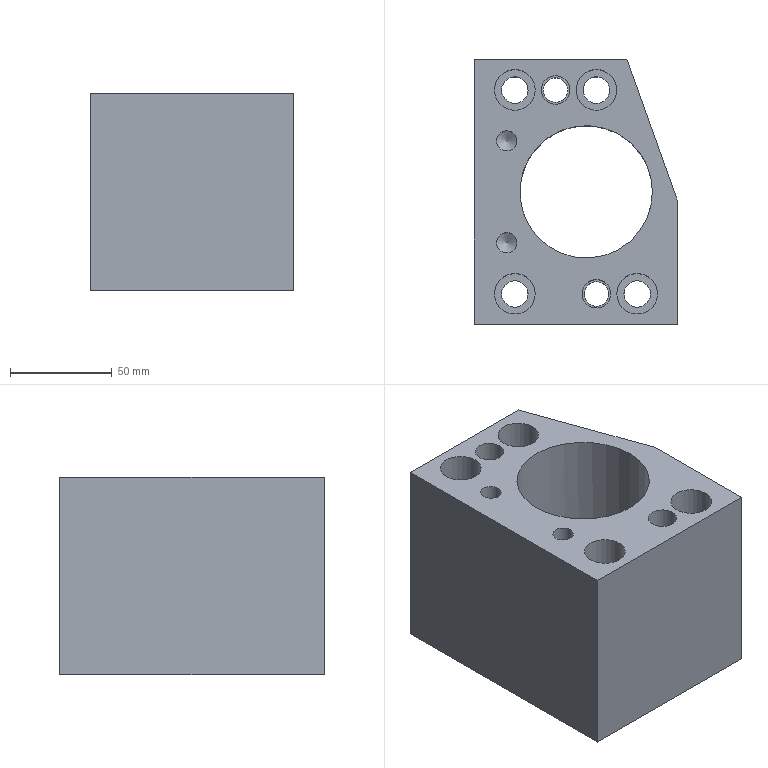Part | NX | features solid 2 | 1 solid | 30 faces | box 100 x 130 x 97 mm | volume 724310 mm3 | cylinder 15 | plane 13 | cone 2 | commonest cylinder face diameters 13 x4 20 x4 10 x2 12 x2 14 x2 65 x1
STEP:
#1=CARTESIAN_POINT('',(-622.,20.,-57.));
#2=VERTEX_POINT('',#1);
#3=CARTESIAN_POINT('',(-615.,20.,-57.));
#4=DIRECTION('',(0.,0.,-1.));
#5=DIRECTION('',(-1.,0.,0.));
#6=AXIS2_PLACEMENT_3D('',#3,#4,#5);
#7=CIRCLE('',#6,7.);
#8=EDGE_CURVE('',#2,#2,#7,.T.);
#9=ORIENTED_EDGE('',*,*,#8,.T.);
#10=EDGE_LOOP('',(#9));
#11=FACE_BOUND('',#10,.T.);
#12=CARTESIAN_POINT('',(-602.,-80.,-57.));
#13=VERTEX_POINT('',#12);
#14=CARTESIAN_POINT('',(-595.,-80.,-57.));
#15=DIRECTION('',(0.,0.,-1.));
#16=DIRECTION('',(-1.,0.,0.));
#17=AXIS2_PLACEMENT_3D('',#14,#15,#16);
#18=CIRCLE('',#17,7.);
#19=EDGE_CURVE('',#13,#13,#18,.T.);
#20=ORIENTED_EDGE('',*,*,#19,.T.);
#21=EDGE_LOOP('',(#20));
#22=FACE_BOUND('',#21,.T.);
#23=CARTESIAN_POINT('',(-645.,-80.,-57.));
#24=VERTEX_POINT('',#23);
#25=CARTESIAN_POINT('',(-635.,-80.,-57.));
#26=DIRECTION('',(0.,0.,-1.));
#27=DIRECTION('',(-1.,0.,0.));
#28=AXIS2_PLACEMENT_3D('',#25,#26,#27);
#29=CIRCLE('',#28,10.);
#30=EDGE_CURVE('',#24,#24,#29,.T.);
#31=ORIENTED_EDGE('',*,*,#30,.T.);
#32=EDGE_LOOP('',(#31));
#33=FACE_BOUND('',#32,.T.);
#34=CARTESIAN_POINT('',(-585.,-80.,-57.));
#35=VERTEX_POINT('',#34);
#36=CARTESIAN_POINT('',(-575.,-80.,-57.));
#37=DIRECTION('',(0.,0.,-1.));
#38=DIRECTION('',(-1.,0.,0.));
#39=AXIS2_PLACEMENT_3D('',#36,#37,#38);
#40=CIRCLE('',#39,10.);
#41=EDGE_CURVE('',#35,#35,#40,.T.);
#42=ORIENTED_EDGE('',*,*,#41,.T.);
#43=EDGE_LOOP('',(#42));
#44=FACE_BOUND('',#43,.T.);
#45=CARTESIAN_POINT('',(-605.,20.,-57.));
#46=VERTEX_POINT('',#45);
#47=CARTESIAN_POINT('',(-595.,20.,-57.));
#48=DIRECTION('',(0.,0.,-1.));
#49=DIRECTION('',(-1.,0.,0.));
#50=AXIS2_PLACEMENT_3D('',#47,#48,#49);
#51=CIRCLE('',#50,10.);
#52=EDGE_CURVE('',#46,#46,#51,.T.);
#53=ORIENTED_EDGE('',*,*,#52,.T.);
#54=EDGE_LOOP('',(#53));
#55=FACE_BOUND('',#54,.T.);
#56=CARTESIAN_POINT('',(-645.,20.,-57.));
#57=VERTEX_POINT('',#56);
#58=CARTESIAN_POINT('',(-635.,20.,-57.));
#59=DIRECTION('',(0.,0.,-1.));
#60=DIRECTION('',(-1.,0.,0.));
#61=AXIS2_PLACEMENT_3D('',#58,#59,#60);
#62=CIRCLE('',#61,10.);
#63=EDGE_CURVE('',#57,#57,#62,.T.);
#64=ORIENTED_EDGE('',*,*,#63,.T.);
#65=EDGE_LOOP('',(#64));
#66=FACE_BOUND('',#65,.T.);
#67=CARTESIAN_POINT('',(-567.5,-30.,-57.));
#68=VERTEX_POINT('',#67);
#69=CARTESIAN_POINT('',(-600.,-30.,-57.));
#70=DIRECTION('',(0.,0.,1.));
#71=DIRECTION('',(1.,0.,0.));
#72=AXIS2_PLACEMENT_3D('',#69,#70,#71);
#73=CIRCLE('',#72,32.5);
#74=EDGE_CURVE('',#68,#68,#73,.T.);
#75=ORIENTED_EDGE('',*,*,#74,.F.);
#76=EDGE_LOOP('',(#75));
#77=FACE_BOUND('',#76,.T.);
#78=CARTESIAN_POINT('',(-644.,-5.,-57.));
#79=VERTEX_POINT('',#78);
#80=CARTESIAN_POINT('',(-639.,-5.,-57.));
#81=DIRECTION('',(0.,0.,-1.));
#82=DIRECTION('',(-1.,0.,0.));
#83=AXIS2_PLACEMENT_3D('',#80,#81,#82);
#84=CIRCLE('',#83,5.);
#85=EDGE_CURVE('',#79,#79,#84,.T.);
#86=ORIENTED_EDGE('',*,*,#85,.T.);
#87=EDGE_LOOP('',(#86));
#88=FACE_BOUND('',#87,.T.);
#89=CARTESIAN_POINT('',(-644.,-55.,-57.));
#90=VERTEX_POINT('',#89);
#91=CARTESIAN_POINT('',(-639.,-55.,-57.));
#92=DIRECTION('',(0.,0.,-1.));
#93=DIRECTION('',(-1.,0.,0.));
#94=AXIS2_PLACEMENT_3D('',#91,#92,#93);
#95=CIRCLE('',#94,5.);
#96=EDGE_CURVE('',#90,#90,#95,.T.);
#97=ORIENTED_EDGE('',*,*,#96,.T.);
#98=EDGE_LOOP('',(#97));
#99=FACE_BOUND('',#98,.T.);
#100=CARTESIAN_POINT('',(-580.,35.,-57.));
#101=VERTEX_POINT('',#100);
#102=CARTESIAN_POINT('',(-555.,-35.,-57.));
#103=VERTEX_POINT('',#102);
#104=CARTESIAN_POINT('',(-551.833,-43.869,-57.));
#105=DIRECTION('',(0.3363,-0.9417,0.));
#106=VECTOR('',#105,1000.);
#107=LINE('',#104,#106);
#108=EDGE_CURVE('',#101,#103,#107,.T.);
#109=ORIENTED_EDGE('',*,*,#108,.F.);
#110=CARTESIAN_POINT('',(-655.,35.,-57.));
#111=VERTEX_POINT('',#110);
#112=CARTESIAN_POINT('',(-555.,35.,-57.));
#113=DIRECTION('',(-1.,0.,0.));
#114=VECTOR('',#113,1000.);
#115=LINE('',#112,#114);
#116=EDGE_CURVE('',#101,#111,#115,.T.);
#117=ORIENTED_EDGE('',*,*,#116,.T.);
#118=CARTESIAN_POINT('',(-655.,-95.,-57.));
#119=VERTEX_POINT('',#118);
#120=CARTESIAN_POINT('',(-655.,35.,-57.));
#121=DIRECTION('',(0.,-1.,0.));
#122=VECTOR('',#121,1000.);
#123=LINE('',#120,#122);
#124=EDGE_CURVE('',#111,#119,#123,.T.);
#125=ORIENTED_EDGE('',*,*,#124,.T.);
#126=CARTESIAN_POINT('',(-555.,-95.,-57.));
#127=VERTEX_POINT('',#126);
#128=CARTESIAN_POINT('',(-625.,-95.,-57.));
#129=DIRECTION('',(1.,0.,0.));
#130=VECTOR('',#129,1000.);
#131=LINE('',#128,#130);
#132=EDGE_CURVE('',#127,#119,#131,.F.);
#133=ORIENTED_EDGE('',*,*,#132,.F.);
#134=CARTESIAN_POINT('',(-555.,35.,-57.));
#135=DIRECTION('',(0.,-1.,0.));
#136=VECTOR('',#135,1000.);
#137=LINE('',#134,#136);
#138=EDGE_CURVE('',#103,#127,#137,.T.);
#139=ORIENTED_EDGE('',*,*,#138,.F.);
#140=EDGE_LOOP('',(#109,#117,#125,#133,#139));
#141=FACE_BOUND('',#140,.T.);
#142=CARTESIAN_POINT('',(-625.,-70.,-57.));
#143=DIRECTION('',(0.,0.,-1.));
#144=DIRECTION('',(0.,1.,0.));
#145=AXIS2_PLACEMENT_3D('',#142,#143,#144);
#146=PLANE('',#145);
#147=ADVANCED_FACE('',(#11,#22,#33,#44,#55,#66,#77,#88,#99,#141),#146,.F.);
#148=CARTESIAN_POINT('',(-609.,20.,-154.));
#149=VERTEX_POINT('',#148);
#150=CARTESIAN_POINT('',(-615.,20.,-154.));
#151=DIRECTION('',(0.,0.,1.));
#152=DIRECTION('',(1.,0.,0.));
#153=AXIS2_PLACEMENT_3D('',#150,#151,#152);
#154=CIRCLE('',#153,6.);
#155=EDGE_CURVE('',#149,#149,#154,.F.);
#156=ORIENTED_EDGE('',*,*,#155,.F.);
#157=EDGE_LOOP('',(#156));
#158=FACE_BOUND('',#157,.T.);
#159=CARTESIAN_POINT('',(-628.5,-80.,-154.));
#160=VERTEX_POINT('',#159);
#161=CARTESIAN_POINT('',(-635.,-80.,-154.));
#162=DIRECTION('',(0.,0.,1.));
#163=DIRECTION('',(1.,0.,0.));
#164=AXIS2_PLACEMENT_3D('',#161,#162,#163);
#165=CIRCLE('',#164,6.5);
#166=EDGE_CURVE('',#160,#160,#165,.T.);
#167=ORIENTED_EDGE('',*,*,#166,.T.);
#168=EDGE_LOOP('',(#167));
#169=FACE_BOUND('',#168,.T.);
#170=CARTESIAN_POINT('',(-568.5,-80.,-154.));
#171=VERTEX_POINT('',#170);
#172=CARTESIAN_POINT('',(-575.,-80.,-154.));
#173=DIRECTION('',(0.,0.,1.));
#174=DIRECTION('',(1.,0.,0.));
#175=AXIS2_PLACEMENT_3D('',#172,#173,#174);
#176=CIRCLE('',#175,6.5);
#177=EDGE_CURVE('',#171,#171,#176,.T.);
#178=ORIENTED_EDGE('',*,*,#177,.T.);
#179=EDGE_LOOP('',(#178));
#180=FACE_BOUND('',#179,.T.);
#181=CARTESIAN_POINT('',(-588.5,20.,-154.));
#182=VERTEX_POINT('',#181);
#183=CARTESIAN_POINT('',(-595.,20.,-154.));
#184=DIRECTION('',(0.,0.,1.));
#185=DIRECTION('',(1.,0.,0.));
#186=AXIS2_PLACEMENT_3D('',#183,#184,#185);
#187=CIRCLE('',#186,6.5);
#188=EDGE_CURVE('',#182,#182,#187,.T.);
#189=ORIENTED_EDGE('',*,*,#188,.T.);
#190=EDGE_LOOP('',(#189));
#191=FACE_BOUND('',#190,.T.);
#192=CARTESIAN_POINT('',(-628.5,20.,-154.));
#193=VERTEX_POINT('',#192);
#194=CARTESIAN_POINT('',(-635.,20.,-154.));
#195=DIRECTION('',(0.,0.,1.));
#196=DIRECTION('',(1.,0.,0.));
#197=AXIS2_PLACEMENT_3D('',#194,#195,#196);
#198=CIRCLE('',#197,6.5);
#199=EDGE_CURVE('',#193,#193,#198,.T.);
#200=ORIENTED_EDGE('',*,*,#199,.T.);
#201=EDGE_LOOP('',(#200));
#202=FACE_BOUND('',#201,.T.);
#203=CARTESIAN_POINT('',(-632.5,-30.,-154.));
#204=VERTEX_POINT('',#203);
#205=CARTESIAN_POINT('',(-600.,-30.,-154.));
#206=DIRECTION('',(0.,0.,1.));
#207=DIRECTION('',(-1.,0.,0.));
#208=AXIS2_PLACEMENT_3D('',#205,#206,#207);
#209=CIRCLE('',#208,32.5);
#210=EDGE_CURVE('',#204,#204,#209,.T.);
#211=ORIENTED_EDGE('',*,*,#210,.T.);
#212=EDGE_LOOP('',(#211));
#213=FACE_BOUND('',#212,.T.);
#214=CARTESIAN_POINT('',(-580.,35.,-154.));
#215=VERTEX_POINT('',#214);
#216=CARTESIAN_POINT('',(-655.,35.,-154.));
#217=VERTEX_POINT('',#216);
#218=CARTESIAN_POINT('',(-555.,35.,-154.));
#219=DIRECTION('',(-1.,0.,0.));
#220=VECTOR('',#219,1000.);
#221=LINE('',#218,#220);
#222=EDGE_CURVE('',#215,#217,#221,.T.);
#223=ORIENTED_EDGE('',*,*,#222,.F.);
#224=CARTESIAN_POINT('',(-555.,-35.,-154.));
#225=VERTEX_POINT('',#224);
#226=CARTESIAN_POINT('',(-555.,-35.,-154.));
#227=DIRECTION('',(0.3363,-0.9417,0.));
#228=VECTOR('',#227,1000.);
#229=LINE('',#226,#228);
#230=EDGE_CURVE('',#215,#225,#229,.T.);
#231=ORIENTED_EDGE('',*,*,#230,.T.);
#232=CARTESIAN_POINT('',(-555.,-95.,-154.));
#233=VERTEX_POINT('',#232);
#234=CARTESIAN_POINT('',(-555.,35.,-154.));
#235=DIRECTION('',(0.,-1.,0.));
#236=VECTOR('',#235,1000.);
#237=LINE('',#234,#236);
#238=EDGE_CURVE('',#225,#233,#237,.T.);
#239=ORIENTED_EDGE('',*,*,#238,.T.);
#240=CARTESIAN_POINT('',(-655.,-95.,-154.));
#241=VERTEX_POINT('',#240);
#242=CARTESIAN_POINT('',(-555.,-95.,-154.));
#243=DIRECTION('',(-1.,0.,0.));
#244=VECTOR('',#243,1000.);
#245=LINE('',#242,#244);
#246=EDGE_CURVE('',#241,#233,#245,.F.);
#247=ORIENTED_EDGE('',*,*,#246,.F.);
#248=CARTESIAN_POINT('',(-655.,35.,-154.));
#249=DIRECTION('',(0.,-1.,0.));
#250=VECTOR('',#249,1000.);
#251=LINE('',#248,#250);
#252=EDGE_CURVE('',#217,#241,#251,.T.);
#253=ORIENTED_EDGE('',*,*,#252,.F.);
#254=EDGE_LOOP('',(#223,#231,#239,#247,#253));
#255=FACE_BOUND('',#254,.T.);
#256=CARTESIAN_POINT('',(-589.,-80.,-154.));
#257=VERTEX_POINT('',#256);
#258=CARTESIAN_POINT('',(-595.,-80.,-154.));
#259=DIRECTION('',(0.,0.,1.));
#260=DIRECTION('',(1.,0.,0.));
#261=AXIS2_PLACEMENT_3D('',#258,#259,#260);
#262=CIRCLE('',#261,6.);
#263=EDGE_CURVE('',#257,#257,#262,.F.);
#264=ORIENTED_EDGE('',*,*,#263,.F.);
#265=EDGE_LOOP('',(#264));
#266=FACE_BOUND('',#265,.T.);
#267=CARTESIAN_POINT('',(-655.,-125.,-154.));
#268=DIRECTION('',(0.,0.,1.));
#269=DIRECTION('',(1.,0.,0.));
#270=AXIS2_PLACEMENT_3D('',#267,#268,#269);
#271=PLANE('',#270);
#272=ADVANCED_FACE('',(#158,#169,#180,#191,#202,#213,#255,#266),#271,.F.);
#273=ORIENTED_EDGE('',*,*,#116,.F.);
#274=CARTESIAN_POINT('',(-580.,35.,-160.));
#275=DIRECTION('',(0.,0.,1.));
#276=VECTOR('',#275,1000.);
#277=LINE('',#274,#276);
#278=EDGE_CURVE('',#215,#101,#277,.T.);
#279=ORIENTED_EDGE('',*,*,#278,.F.);
#280=ORIENTED_EDGE('',*,*,#222,.T.);
#281=CARTESIAN_POINT('',(-655.,35.,-160.));
#282=DIRECTION('',(0.,0.,1.));
#283=VECTOR('',#282,1000.);
#284=LINE('',#281,#283);
#285=EDGE_CURVE('',#217,#111,#284,.T.);
#286=ORIENTED_EDGE('',*,*,#285,.T.);
#287=EDGE_LOOP('',(#273,#279,#280,#286));
#288=FACE_BOUND('',#287,.T.);
#289=CARTESIAN_POINT('',(-555.,35.,-160.));
#290=DIRECTION('',(0.,-1.,0.));
#291=DIRECTION('',(0.,0.,1.));
#292=AXIS2_PLACEMENT_3D('',#289,#290,#291);
#293=PLANE('',#292);
#294=ADVANCED_FACE('',(#288),#293,.F.);
#295=ORIENTED_EDGE('',*,*,#238,.F.);
#296=CARTESIAN_POINT('',(-555.,-35.,-160.));
#297=DIRECTION('',(0.,0.,1.));
#298=VECTOR('',#297,1000.);
#299=LINE('',#296,#298);
#300=EDGE_CURVE('',#225,#103,#299,.T.);
#301=ORIENTED_EDGE('',*,*,#300,.T.);
#302=ORIENTED_EDGE('',*,*,#138,.T.);
#303=CARTESIAN_POINT('',(-555.,-95.,-160.));
#304=DIRECTION('',(0.,0.,1.));
#305=VECTOR('',#304,1000.);
#306=LINE('',#303,#305);
#307=EDGE_CURVE('',#233,#127,#306,.T.);
#308=ORIENTED_EDGE('',*,*,#307,.F.);
#309=EDGE_LOOP('',(#295,#301,#302,#308));
#310=FACE_BOUND('',#309,.T.);
#311=CARTESIAN_POINT('',(-555.,35.,-160.));
#312=DIRECTION('',(1.,0.,0.));
#313=DIRECTION('',(0.,0.,1.));
#314=AXIS2_PLACEMENT_3D('',#311,#312,#313);
#315=PLANE('',#314);
#316=ADVANCED_FACE('',(#310),#315,.T.);
#317=CARTESIAN_POINT('',(-655.,-95.,-160.));
#318=DIRECTION('',(0.,0.,1.));
#319=VECTOR('',#318,1000.);
#320=LINE('',#317,#319);
#321=EDGE_CURVE('',#241,#119,#320,.T.);
#322=ORIENTED_EDGE('',*,*,#321,.F.);
#323=ORIENTED_EDGE('',*,*,#246,.T.);
#324=ORIENTED_EDGE('',*,*,#307,.T.);
#325=ORIENTED_EDGE('',*,*,#132,.T.);
#326=EDGE_LOOP('',(#322,#323,#324,#325));
#327=FACE_BOUND('',#326,.T.);
#328=CARTESIAN_POINT('',(-555.,-95.,-160.));
#329=DIRECTION('',(0.,-1.,0.));
#330=DIRECTION('',(0.,0.,1.));
#331=AXIS2_PLACEMENT_3D('',#328,#329,#330);
#332=PLANE('',#331);
#333=ADVANCED_FACE('',(#327),#332,.T.);
#334=ORIENTED_EDGE('',*,*,#285,.F.);
#335=ORIENTED_EDGE('',*,*,#252,.T.);
#336=ORIENTED_EDGE('',*,*,#321,.T.);
#337=ORIENTED_EDGE('',*,*,#124,.F.);
#338=EDGE_LOOP('',(#334,#335,#336,#337));
#339=FACE_BOUND('',#338,.T.);
#340=CARTESIAN_POINT('',(-655.,35.,-160.));
#341=DIRECTION('',(1.,0.,0.));
#342=DIRECTION('',(0.,0.,1.));
#343=AXIS2_PLACEMENT_3D('',#340,#341,#342);
#344=PLANE('',#343);
#345=ADVANCED_FACE('',(#339),#344,.F.);
#346=ORIENTED_EDGE('',*,*,#210,.F.);
#347=EDGE_LOOP('',(#346));
#348=FACE_BOUND('',#347,.T.);
#349=ORIENTED_EDGE('',*,*,#74,.T.);
#350=EDGE_LOOP('',(#349));
#351=FACE_BOUND('',#350,.T.);
#352=CARTESIAN_POINT('',(-600.,-30.,-49.));
#353=DIRECTION('',(0.,0.,-1.));
#354=DIRECTION('',(1.,0.,0.));
#355=AXIS2_PLACEMENT_3D('',#352,#353,#354);
#356=CYLINDRICAL_SURFACE('',#355,32.5);
#357=ADVANCED_FACE('',(#348,#351),#356,.F.);
#358=CARTESIAN_POINT('',(-644.,-5.,-97.));
#359=VERTEX_POINT('',#358);
#360=CARTESIAN_POINT('',(-639.,-5.,-97.));
#361=DIRECTION('',(0.,0.,-1.));
#362=DIRECTION('',(-1.,0.,0.));
#363=AXIS2_PLACEMENT_3D('',#360,#361,#362);
#364=CIRCLE('',#363,5.);
#365=EDGE_CURVE('',#359,#359,#364,.T.);
#366=ORIENTED_EDGE('',*,*,#365,.F.);
#367=EDGE_LOOP('',(#366));
#368=FACE_BOUND('',#367,.T.);
#369=CARTESIAN_POINT('',(-639.,-5.,-100.004));
#370=VERTEX_POINT('',#369);
#371=VERTEX_LOOP('',#370);
#372=FACE_BOUND('',#371,.T.);
#373=CARTESIAN_POINT('',(-639.,-5.,-97.));
#374=DIRECTION('',(0.,0.,1.));
#375=DIRECTION('',(1.,0.,0.));
#376=AXIS2_PLACEMENT_3D('',#373,#374,#375);
#377=CONICAL_SURFACE('',#376,5.,1.03);
#378=ADVANCED_FACE('',(#368,#372),#377,.F.);
#379=ORIENTED_EDGE('',*,*,#365,.T.);
#380=EDGE_LOOP('',(#379));
#381=FACE_BOUND('',#380,.T.);
#382=ORIENTED_EDGE('',*,*,#85,.F.);
#383=EDGE_LOOP('',(#382));
#384=FACE_BOUND('',#383,.T.);
#385=CARTESIAN_POINT('',(-639.,-5.,-57.));
#386=DIRECTION('',(0.,0.,-1.));
#387=DIRECTION('',(-1.,0.,0.));
#388=AXIS2_PLACEMENT_3D('',#385,#386,#387);
#389=CYLINDRICAL_SURFACE('',#388,5.);
#390=ADVANCED_FACE('',(#381,#384),#389,.F.);
#391=CARTESIAN_POINT('',(-644.,-55.,-97.));
#392=VERTEX_POINT('',#391);
#393=CARTESIAN_POINT('',(-639.,-55.,-97.));
#394=DIRECTION('',(0.,0.,-1.));
#395=DIRECTION('',(-1.,0.,0.));
#396=AXIS2_PLACEMENT_3D('',#393,#394,#395);
#397=CIRCLE('',#396,5.);
#398=EDGE_CURVE('',#392,#392,#397,.T.);
#399=ORIENTED_EDGE('',*,*,#398,.F.);
#400=EDGE_LOOP('',(#399));
#401=FACE_BOUND('',#400,.T.);
#402=CARTESIAN_POINT('',(-639.,-55.,-100.004));
#403=VERTEX_POINT('',#402);
#404=VERTEX_LOOP('',#403);
#405=FACE_BOUND('',#404,.T.);
#406=CARTESIAN_POINT('',(-639.,-55.,-97.));
#407=DIRECTION('',(0.,0.,1.));
#408=DIRECTION('',(1.,0.,0.));
#409=AXIS2_PLACEMENT_3D('',#406,#407,#408);
#410=CONICAL_SURFACE('',#409,5.,1.03);
#411=ADVANCED_FACE('',(#401,#405),#410,.F.);
#412=ORIENTED_EDGE('',*,*,#398,.T.);
#413=EDGE_LOOP('',(#412));
#414=FACE_BOUND('',#413,.T.);
#415=ORIENTED_EDGE('',*,*,#96,.F.);
#416=EDGE_LOOP('',(#415));
#417=FACE_BOUND('',#416,.T.);
#418=CARTESIAN_POINT('',(-639.,-55.,-57.));
#419=DIRECTION('',(0.,0.,-1.));
#420=DIRECTION('',(-1.,0.,0.));
#421=AXIS2_PLACEMENT_3D('',#418,#419,#420);
#422=CYLINDRICAL_SURFACE('',#421,5.);
#423=ADVANCED_FACE('',(#414,#417),#422,.F.);
#424=ORIENTED_EDGE('',*,*,#230,.F.);
#425=ORIENTED_EDGE('',*,*,#278,.T.);
#426=ORIENTED_EDGE('',*,*,#108,.T.);
#427=ORIENTED_EDGE('',*,*,#300,.F.);
#428=EDGE_LOOP('',(#424,#425,#426,#427));
#429=FACE_BOUND('',#428,.T.);
#430=CARTESIAN_POINT('',(-555.,-35.,-57.));
#431=DIRECTION('',(0.9417,0.3363,0.));
#432=DIRECTION('',(-0.3363,0.9417,0.));
#433=AXIS2_PLACEMENT_3D('',#430,#431,#432);
#434=PLANE('',#433);
#435=ADVANCED_FACE('',(#429),#434,.T.);
#436=CARTESIAN_POINT('',(-625.,20.,-119.));
#437=VERTEX_POINT('',#436);
#438=CARTESIAN_POINT('',(-635.,20.,-119.));
#439=DIRECTION('',(0.,0.,1.));
#440=DIRECTION('',(1.,0.,0.));
#441=AXIS2_PLACEMENT_3D('',#438,#439,#440);
#442=CIRCLE('',#441,10.);
#443=EDGE_CURVE('',#437,#437,#442,.T.);
#444=ORIENTED_EDGE('',*,*,#443,.F.);
#445=EDGE_LOOP('',(#444));
#446=FACE_BOUND('',#445,.T.);
#447=ORIENTED_EDGE('',*,*,#63,.F.);
#448=EDGE_LOOP('',(#447));
#449=FACE_BOUND('',#448,.T.);
#450=CARTESIAN_POINT('',(-635.,20.,-119.));
#451=DIRECTION('',(0.,0.,1.));
#452=DIRECTION('',(1.,0.,0.));
#453=AXIS2_PLACEMENT_3D('',#450,#451,#452);
#454=CYLINDRICAL_SURFACE('',#453,10.);
#455=ADVANCED_FACE('',(#446,#449),#454,.F.);
#456=CARTESIAN_POINT('',(-641.5,20.,-119.));
#457=VERTEX_POINT('',#456);
#458=CARTESIAN_POINT('',(-635.,20.,-119.));
#459=DIRECTION('',(0.,0.,-1.));
#460=DIRECTION('',(-1.,0.,0.));
#461=AXIS2_PLACEMENT_3D('',#458,#459,#460);
#462=CIRCLE('',#461,6.5);
#463=EDGE_CURVE('',#457,#457,#462,.F.);
#464=ORIENTED_EDGE('',*,*,#463,.T.);
#465=EDGE_LOOP('',(#464));
#466=FACE_BOUND('',#465,.T.);
#467=ORIENTED_EDGE('',*,*,#199,.F.);
#468=EDGE_LOOP('',(#467));
#469=FACE_BOUND('',#468,.T.);
#470=CARTESIAN_POINT('',(-635.,20.,-189.));
#471=DIRECTION('',(0.,0.,1.));
#472=DIRECTION('',(1.,0.,0.));
#473=AXIS2_PLACEMENT_3D('',#470,#471,#472);
#474=CYLINDRICAL_SURFACE('',#473,6.5);
#475=ADVANCED_FACE('',(#466,#469),#474,.F.);
#476=ORIENTED_EDGE('',*,*,#463,.F.);
#477=EDGE_LOOP('',(#476));
#478=FACE_BOUND('',#477,.T.);
#479=ORIENTED_EDGE('',*,*,#443,.T.);
#480=EDGE_LOOP('',(#479));
#481=FACE_BOUND('',#480,.T.);
#482=CARTESIAN_POINT('',(-635.,20.,-119.));
#483=DIRECTION('',(0.,0.,-1.));
#484=DIRECTION('',(-1.,0.,0.));
#485=AXIS2_PLACEMENT_3D('',#482,#483,#484);
#486=PLANE('',#485);
#487=ADVANCED_FACE('',(#478,#481),#486,.F.);
#488=CARTESIAN_POINT('',(-585.,20.,-119.));
#489=VERTEX_POINT('',#488);
#490=CARTESIAN_POINT('',(-595.,20.,-119.));
#491=DIRECTION('',(0.,0.,1.));
#492=DIRECTION('',(1.,0.,0.));
#493=AXIS2_PLACEMENT_3D('',#490,#491,#492);
#494=CIRCLE('',#493,10.);
#495=EDGE_CURVE('',#489,#489,#494,.T.);
#496=ORIENTED_EDGE('',*,*,#495,.F.);
#497=EDGE_LOOP('',(#496));
#498=FACE_BOUND('',#497,.T.);
#499=ORIENTED_EDGE('',*,*,#52,.F.);
#500=EDGE_LOOP('',(#499));
#501=FACE_BOUND('',#500,.T.);
#502=CARTESIAN_POINT('',(-595.,20.,-119.));
#503=DIRECTION('',(0.,0.,1.));
#504=DIRECTION('',(1.,0.,0.));
#505=AXIS2_PLACEMENT_3D('',#502,#503,#504);
#506=CYLINDRICAL_SURFACE('',#505,10.);
#507=ADVANCED_FACE('',(#498,#501),#506,.F.);
#508=CARTESIAN_POINT('',(-601.5,20.,-119.));
#509=VERTEX_POINT('',#508);
#510=CARTESIAN_POINT('',(-595.,20.,-119.));
#511=DIRECTION('',(0.,0.,-1.));
#512=DIRECTION('',(-1.,0.,0.));
#513=AXIS2_PLACEMENT_3D('',#510,#511,#512);
#514=CIRCLE('',#513,6.5);
#515=EDGE_CURVE('',#509,#509,#514,.F.);
#516=ORIENTED_EDGE('',*,*,#515,.T.);
#517=EDGE_LOOP('',(#516));
#518=FACE_BOUND('',#517,.T.);
#519=ORIENTED_EDGE('',*,*,#188,.F.);
#520=EDGE_LOOP('',(#519));
#521=FACE_BOUND('',#520,.T.);
#522=CARTESIAN_POINT('',(-595.,20.,-189.));
#523=DIRECTION('',(0.,0.,1.));
#524=DIRECTION('',(1.,0.,0.));
#525=AXIS2_PLACEMENT_3D('',#522,#523,#524);
#526=CYLINDRICAL_SURFACE('',#525,6.5);
#527=ADVANCED_FACE('',(#518,#521),#526,.F.);
#528=ORIENTED_EDGE('',*,*,#515,.F.);
#529=EDGE_LOOP('',(#528));
#530=FACE_BOUND('',#529,.T.);
#531=ORIENTED_EDGE('',*,*,#495,.T.);
#532=EDGE_LOOP('',(#531));
#533=FACE_BOUND('',#532,.T.);
#534=CARTESIAN_POINT('',(-595.,20.,-119.));
#535=DIRECTION('',(0.,0.,-1.));
#536=DIRECTION('',(-1.,0.,0.));
#537=AXIS2_PLACEMENT_3D('',#534,#535,#536);
#538=PLANE('',#537);
#539=ADVANCED_FACE('',(#530,#533),#538,.F.);
#540=CARTESIAN_POINT('',(-565.,-80.,-119.));
#541=VERTEX_POINT('',#540);
#542=CARTESIAN_POINT('',(-575.,-80.,-119.));
#543=DIRECTION('',(0.,0.,1.));
#544=DIRECTION('',(1.,0.,0.));
#545=AXIS2_PLACEMENT_3D('',#542,#543,#544);
#546=CIRCLE('',#545,10.);
#547=EDGE_CURVE('',#541,#541,#546,.T.);
#548=ORIENTED_EDGE('',*,*,#547,.F.);
#549=EDGE_LOOP('',(#548));
#550=FACE_BOUND('',#549,.T.);
#551=ORIENTED_EDGE('',*,*,#41,.F.);
#552=EDGE_LOOP('',(#551));
#553=FACE_BOUND('',#552,.T.);
#554=CARTESIAN_POINT('',(-575.,-80.,-119.));
#555=DIRECTION('',(0.,0.,1.));
#556=DIRECTION('',(1.,0.,0.));
#557=AXIS2_PLACEMENT_3D('',#554,#555,#556);
#558=CYLINDRICAL_SURFACE('',#557,10.);
#559=ADVANCED_FACE('',(#550,#553),#558,.F.);
#560=CARTESIAN_POINT('',(-581.5,-80.,-119.));
#561=VERTEX_POINT('',#560);
#562=CARTESIAN_POINT('',(-575.,-80.,-119.));
#563=DIRECTION('',(0.,0.,-1.));
#564=DIRECTION('',(-1.,0.,0.));
#565=AXIS2_PLACEMENT_3D('',#562,#563,#564);
#566=CIRCLE('',#565,6.5);
#567=EDGE_CURVE('',#561,#561,#566,.F.);
#568=ORIENTED_EDGE('',*,*,#567,.T.);
#569=EDGE_LOOP('',(#568));
#570=FACE_BOUND('',#569,.T.);
#571=ORIENTED_EDGE('',*,*,#177,.F.);
#572=EDGE_LOOP('',(#571));
#573=FACE_BOUND('',#572,.T.);
#574=CARTESIAN_POINT('',(-575.,-80.,-189.));
#575=DIRECTION('',(0.,0.,1.));
#576=DIRECTION('',(1.,0.,0.));
#577=AXIS2_PLACEMENT_3D('',#574,#575,#576);
#578=CYLINDRICAL_SURFACE('',#577,6.5);
#579=ADVANCED_FACE('',(#570,#573),#578,.F.);
#580=ORIENTED_EDGE('',*,*,#567,.F.);
#581=EDGE_LOOP('',(#580));
#582=FACE_BOUND('',#581,.T.);
#583=ORIENTED_EDGE('',*,*,#547,.T.);
#584=EDGE_LOOP('',(#583));
#585=FACE_BOUND('',#584,.T.);
#586=CARTESIAN_POINT('',(-575.,-80.,-119.));
#587=DIRECTION('',(0.,0.,-1.));
#588=DIRECTION('',(-1.,0.,0.));
#589=AXIS2_PLACEMENT_3D('',#586,#587,#588);
#590=PLANE('',#589);
#591=ADVANCED_FACE('',(#582,#585),#590,.F.);
#592=CARTESIAN_POINT('',(-625.,-80.,-119.));
#593=VERTEX_POINT('',#592);
#594=CARTESIAN_POINT('',(-635.,-80.,-119.));
#595=DIRECTION('',(0.,0.,1.));
#596=DIRECTION('',(1.,0.,0.));
#597=AXIS2_PLACEMENT_3D('',#594,#595,#596);
#598=CIRCLE('',#597,10.);
#599=EDGE_CURVE('',#593,#593,#598,.T.);
#600=ORIENTED_EDGE('',*,*,#599,.F.);
#601=EDGE_LOOP('',(#600));
#602=FACE_BOUND('',#601,.T.);
#603=ORIENTED_EDGE('',*,*,#30,.F.);
#604=EDGE_LOOP('',(#603));
#605=FACE_BOUND('',#604,.T.);
#606=CARTESIAN_POINT('',(-635.,-80.,-119.));
#607=DIRECTION('',(0.,0.,1.));
#608=DIRECTION('',(1.,0.,0.));
#609=AXIS2_PLACEMENT_3D('',#606,#607,#608);
#610=CYLINDRICAL_SURFACE('',#609,10.);
#611=ADVANCED_FACE('',(#602,#605),#610,.F.);
#612=CARTESIAN_POINT('',(-641.5,-80.,-119.));
#613=VERTEX_POINT('',#612);
#614=CARTESIAN_POINT('',(-635.,-80.,-119.));
#615=DIRECTION('',(0.,0.,-1.));
#616=DIRECTION('',(-1.,0.,0.));
#617=AXIS2_PLACEMENT_3D('',#614,#615,#616);
#618=CIRCLE('',#617,6.5);
#619=EDGE_CURVE('',#613,#613,#618,.F.);
#620=ORIENTED_EDGE('',*,*,#619,.T.);
#621=EDGE_LOOP('',(#620));
#622=FACE_BOUND('',#621,.T.);
#623=ORIENTED_EDGE('',*,*,#166,.F.);
#624=EDGE_LOOP('',(#623));
#625=FACE_BOUND('',#624,.T.);
#626=CARTESIAN_POINT('',(-635.,-80.,-189.));
#627=DIRECTION('',(0.,0.,1.));
#628=DIRECTION('',(1.,0.,0.));
#629=AXIS2_PLACEMENT_3D('',#626,#627,#628);
#630=CYLINDRICAL_SURFACE('',#629,6.5);
#631=ADVANCED_FACE('',(#622,#625),#630,.F.);
#632=ORIENTED_EDGE('',*,*,#619,.F.);
#633=EDGE_LOOP('',(#632));
#634=FACE_BOUND('',#633,.T.);
#635=ORIENTED_EDGE('',*,*,#599,.T.);
#636=EDGE_LOOP('',(#635));
#637=FACE_BOUND('',#636,.T.);
#638=CARTESIAN_POINT('',(-635.,-80.,-119.));
#639=DIRECTION('',(0.,0.,-1.));
#640=DIRECTION('',(-1.,0.,0.));
#641=AXIS2_PLACEMENT_3D('',#638,#639,#640);
#642=PLANE('',#641);
#643=ADVANCED_FACE('',(#634,#637),#642,.F.);
#644=CARTESIAN_POINT('',(-621.,20.,-119.));
#645=VERTEX_POINT('',#644);
#646=CARTESIAN_POINT('',(-615.,20.,-119.));
#647=DIRECTION('',(0.,0.,-1.));
#648=DIRECTION('',(-1.,0.,0.));
#649=AXIS2_PLACEMENT_3D('',#646,#647,#648);
#650=CIRCLE('',#649,6.);
#651=EDGE_CURVE('',#645,#645,#650,.T.);
#652=ORIENTED_EDGE('',*,*,#651,.F.);
#653=EDGE_LOOP('',(#652));
#654=FACE_BOUND('',#653,.T.);
#655=ORIENTED_EDGE('',*,*,#155,.T.);
#656=EDGE_LOOP('',(#655));
#657=FACE_BOUND('',#656,.T.);
#658=CARTESIAN_POINT('',(-615.,20.,-319.));
#659=DIRECTION('',(0.,0.,1.));
#660=DIRECTION('',(1.,0.,0.));
#661=AXIS2_PLACEMENT_3D('',#658,#659,#660);
#662=CYLINDRICAL_SURFACE('',#661,6.);
#663=ADVANCED_FACE('',(#654,#657),#662,.F.);
#664=CARTESIAN_POINT('',(-601.,-80.,-119.));
#665=VERTEX_POINT('',#664);
#666=CARTESIAN_POINT('',(-595.,-80.,-119.));
#667=DIRECTION('',(0.,0.,-1.));
#668=DIRECTION('',(-1.,0.,0.));
#669=AXIS2_PLACEMENT_3D('',#666,#667,#668);
#670=CIRCLE('',#669,6.);
#671=EDGE_CURVE('',#665,#665,#670,.T.);
#672=ORIENTED_EDGE('',*,*,#671,.F.);
#673=EDGE_LOOP('',(#672));
#674=FACE_BOUND('',#673,.T.);
#675=ORIENTED_EDGE('',*,*,#263,.T.);
#676=EDGE_LOOP('',(#675));
#677=FACE_BOUND('',#676,.T.);
#678=CARTESIAN_POINT('',(-595.,-80.,-319.));
#679=DIRECTION('',(0.,0.,1.));
#680=DIRECTION('',(1.,0.,0.));
#681=AXIS2_PLACEMENT_3D('',#678,#679,#680);
#682=CYLINDRICAL_SURFACE('',#681,6.);
#683=ADVANCED_FACE('',(#674,#677),#682,.F.);
#684=CARTESIAN_POINT('',(-602.,-80.,-119.));
#685=VERTEX_POINT('',#684);
#686=CARTESIAN_POINT('',(-595.,-80.,-119.));
#687=DIRECTION('',(0.,0.,-1.));
#688=DIRECTION('',(-1.,0.,0.));
#689=AXIS2_PLACEMENT_3D('',#686,#687,#688);
#690=CIRCLE('',#689,7.);
#691=EDGE_CURVE('',#685,#685,#690,.T.);
#692=ORIENTED_EDGE('',*,*,#691,.T.);
#693=EDGE_LOOP('',(#692));
#694=FACE_BOUND('',#693,.T.);
#695=ORIENTED_EDGE('',*,*,#19,.F.);
#696=EDGE_LOOP('',(#695));
#697=FACE_BOUND('',#696,.T.);
#698=CARTESIAN_POINT('',(-595.,-80.,146.));
#699=DIRECTION('',(0.,0.,-1.));
#700=DIRECTION('',(-1.,0.,0.));
#701=AXIS2_PLACEMENT_3D('',#698,#699,#700);
#702=CYLINDRICAL_SURFACE('',#701,7.);
#703=ADVANCED_FACE('',(#694,#697),#702,.F.);
#704=ORIENTED_EDGE('',*,*,#671,.T.);
#705=EDGE_LOOP('',(#704));
#706=FACE_BOUND('',#705,.T.);
#707=ORIENTED_EDGE('',*,*,#691,.F.);
#708=EDGE_LOOP('',(#707));
#709=FACE_BOUND('',#708,.T.);
#710=CARTESIAN_POINT('',(-595.,-80.,-119.));
#711=DIRECTION('',(0.,0.,-1.));
#712=DIRECTION('',(-1.,0.,0.));
#713=AXIS2_PLACEMENT_3D('',#710,#711,#712);
#714=PLANE('',#713);
#715=ADVANCED_FACE('',(#706,#709),#714,.F.);
#716=CARTESIAN_POINT('',(-622.,20.,-119.));
#717=VERTEX_POINT('',#716);
#718=CARTESIAN_POINT('',(-615.,20.,-119.));
#719=DIRECTION('',(0.,0.,-1.));
#720=DIRECTION('',(-1.,0.,0.));
#721=AXIS2_PLACEMENT_3D('',#718,#719,#720);
#722=CIRCLE('',#721,7.);
#723=EDGE_CURVE('',#717,#717,#722,.T.);
#724=ORIENTED_EDGE('',*,*,#723,.T.);
#725=EDGE_LOOP('',(#724));
#726=FACE_BOUND('',#725,.T.);
#727=ORIENTED_EDGE('',*,*,#8,.F.);
#728=EDGE_LOOP('',(#727));
#729=FACE_BOUND('',#728,.T.);
#730=CARTESIAN_POINT('',(-615.,20.,146.));
#731=DIRECTION('',(0.,0.,-1.));
#732=DIRECTION('',(-1.,0.,0.));
#733=AXIS2_PLACEMENT_3D('',#730,#731,#732);
#734=CYLINDRICAL_SURFACE('',#733,7.);
#735=ADVANCED_FACE('',(#726,#729),#734,.F.);
#736=ORIENTED_EDGE('',*,*,#651,.T.);
#737=EDGE_LOOP('',(#736));
#738=FACE_BOUND('',#737,.T.);
#739=ORIENTED_EDGE('',*,*,#723,.F.);
#740=EDGE_LOOP('',(#739));
#741=FACE_BOUND('',#740,.T.);
#742=CARTESIAN_POINT('',(-615.,20.,-119.));
#743=DIRECTION('',(0.,0.,-1.));
#744=DIRECTION('',(-1.,0.,0.));
#745=AXIS2_PLACEMENT_3D('',#742,#743,#744);
#746=PLANE('',#745);
#747=ADVANCED_FACE('',(#738,#741),#746,.F.);
#748=CLOSED_SHELL('',(#147,#272,#294,#316,#333,#345,#357,#378,#390,#411,#423,#435,#455,#475,#487,#507,#527,#539,#559,#579,#591,#611,#631,#643,#663,#683,#703,#715,#735,#747));
#749=MANIFOLD_SOLID_BREP('',#748);
#750=(LENGTH_UNIT()NAMED_UNIT(*)SI_UNIT(.MILLI.,.METRE.));
#751=UNCERTAINTY_MEASURE_WITH_UNIT(LENGTH_MEASURE(0.00001),#750,'','');
#752=(NAMED_UNIT(*)PLANE_ANGLE_UNIT()SI_UNIT($,.RADIAN.));
#753=(NAMED_UNIT(*)SI_UNIT($,.STERADIAN.)SOLID_ANGLE_UNIT());
#754=(GEOMETRIC_REPRESENTATION_CONTEXT(3)GLOBAL_UNCERTAINTY_ASSIGNED_CONTEXT((#751))GLOBAL_UNIT_ASSIGNED_CONTEXT((#750,#752,#753))REPRESENTATION_CONTEXT('',''));
#755=ADVANCED_BREP_SHAPE_REPRESENTATION('',(#749),#754);